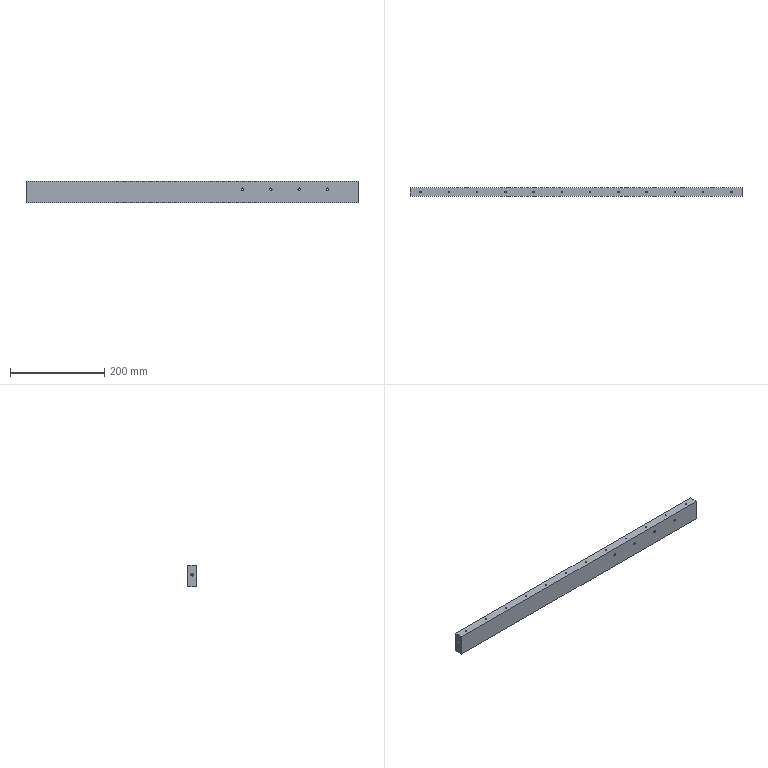Part | STEP file | PN_0086 guide rail spacer block | 1 solid | 146 faces | box 705 x 18 x 45 mm | volume 564305 mm3 | cylinder 74 | cone 66 | plane 6 | commonest cylinder face diameters 5 x34 3.3 x24 2.5 x16